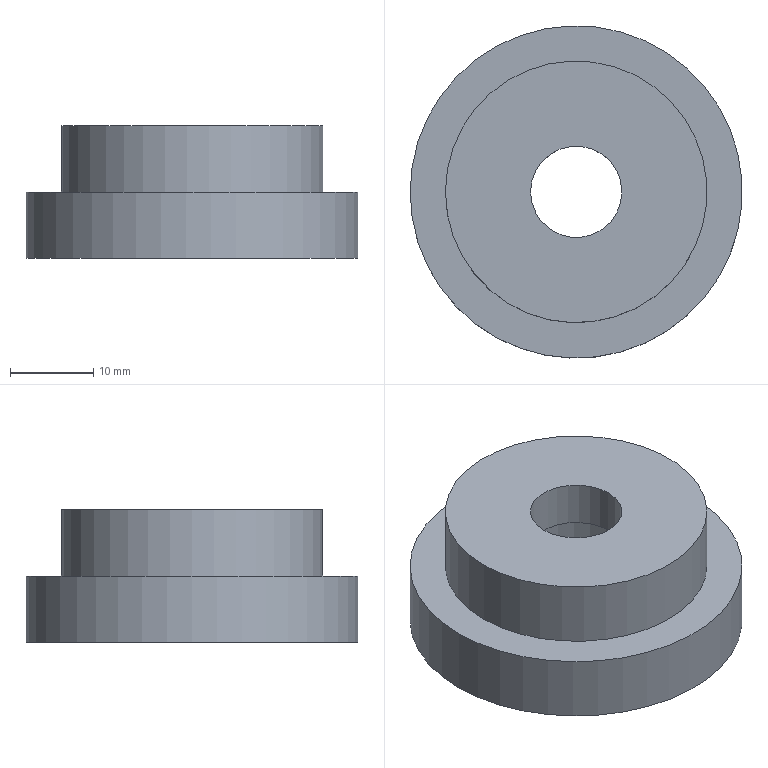Part | STEP file | PN_0057_id1206_x_t | 1 solid | 8 faces | box 40 x 40 x 16 mm | volume 13382 mm3 | cylinder 4 | plane 4 | commonest cylinder face diameters 11 x1 17 x1 31.5 x1 40 x1
STEP:
#1=CARTESIAN_POINT('',(232.,152.5,35.5));
#2=VERTEX_POINT('',#1);
#3=CARTESIAN_POINT('',(237.5,152.5,35.5));
#4=DIRECTION('',(0.,0.,-1.));
#5=DIRECTION('',(-1.,0.,0.));
#6=AXIS2_PLACEMENT_3D('',#3,#4,#5);
#7=CIRCLE('',#6,5.5);
#8=EDGE_CURVE('',#2,#2,#7,.T.);
#9=ORIENTED_EDGE('',*,*,#8,.T.);
#10=CARTESIAN_POINT('',(232.,152.5,41.));
#11=VERTEX_POINT('',#10);
#12=CARTESIAN_POINT('',(232.,152.5,35.5));
#13=CARTESIAN_POINT('',(232.,152.5,41.));
#14=B_SPLINE_CURVE_WITH_KNOTS('',1,(#12,#13),.UNSPECIFIED.,.F.,.F.,(2,2),(0.,1.),.UNSPECIFIED.);
#15=EDGE_CURVE('',#2,#11,#14,.T.);
#16=ORIENTED_EDGE('',*,*,#15,.T.);
#17=CARTESIAN_POINT('',(237.5,152.5,41.));
#18=DIRECTION('',(0.,0.,1.));
#19=DIRECTION('',(-1.,0.,0.));
#20=AXIS2_PLACEMENT_3D('',#17,#18,#19);
#21=CIRCLE('',#20,5.5);
#22=EDGE_CURVE('',#11,#11,#21,.T.);
#23=ORIENTED_EDGE('',*,*,#22,.T.);
#24=ORIENTED_EDGE('',*,*,#15,.F.);
#25=EDGE_LOOP('',(#9,#16,#23,#24));
#26=FACE_OUTER_BOUND('',#25,.T.);
#27=CARTESIAN_POINT('',(237.5,152.5,38.25));
#28=DIRECTION('',(0.,0.,1.));
#29=DIRECTION('',(-1.,0.,0.));
#30=AXIS2_PLACEMENT_3D('',#27,#28,#29);
#31=CYLINDRICAL_SURFACE('',#30,5.5);
#32=ADVANCED_FACE('',(#26),#31,.F.);
#33=CARTESIAN_POINT('',(229.,152.5,25.));
#34=VERTEX_POINT('',#33);
#35=CARTESIAN_POINT('',(237.5,152.5,25.));
#36=DIRECTION('',(0.,0.,-1.));
#37=DIRECTION('',(-1.,0.,0.));
#38=AXIS2_PLACEMENT_3D('',#35,#36,#37);
#39=CIRCLE('',#38,8.5);
#40=EDGE_CURVE('',#34,#34,#39,.T.);
#41=ORIENTED_EDGE('',*,*,#40,.T.);
#42=CARTESIAN_POINT('',(229.,152.5,35.5));
#43=VERTEX_POINT('',#42);
#44=CARTESIAN_POINT('',(229.,152.5,25.));
#45=CARTESIAN_POINT('',(229.,152.5,35.5));
#46=B_SPLINE_CURVE_WITH_KNOTS('',1,(#44,#45),.UNSPECIFIED.,.F.,.F.,(2,2),(0.,1.),.UNSPECIFIED.);
#47=EDGE_CURVE('',#34,#43,#46,.T.);
#48=ORIENTED_EDGE('',*,*,#47,.T.);
#49=CARTESIAN_POINT('',(237.5,152.5,35.5));
#50=DIRECTION('',(0.,0.,-1.));
#51=DIRECTION('',(-1.,0.,0.));
#52=AXIS2_PLACEMENT_3D('',#49,#50,#51);
#53=CIRCLE('',#52,8.5);
#54=EDGE_CURVE('',#43,#43,#53,.T.);
#55=ORIENTED_EDGE('',*,*,#54,.F.);
#56=ORIENTED_EDGE('',*,*,#47,.F.);
#57=EDGE_LOOP('',(#41,#48,#55,#56));
#58=FACE_OUTER_BOUND('',#57,.T.);
#59=CARTESIAN_POINT('',(237.5,152.5,30.25));
#60=DIRECTION('',(0.,0.,1.));
#61=DIRECTION('',(-1.,0.,0.));
#62=AXIS2_PLACEMENT_3D('',#59,#60,#61);
#63=CYLINDRICAL_SURFACE('',#62,8.5);
#64=ADVANCED_FACE('',(#58),#63,.F.);
#65=ORIENTED_EDGE('',*,*,#54,.T.);
#66=EDGE_LOOP('',(#65));
#67=FACE_BOUND('',#66,.T.);
#68=ORIENTED_EDGE('',*,*,#8,.F.);
#69=EDGE_LOOP('',(#68));
#70=FACE_BOUND('',#69,.T.);
#71=CARTESIAN_POINT('',(257.05,134.833,35.5));
#72=DIRECTION('',(0.,0.,1.));
#73=DIRECTION('',(-1.,0.,0.));
#74=AXIS2_PLACEMENT_3D('',#71,#72,#73);
#75=PLANE('',#74);
#76=ADVANCED_FACE('',(#67,#70),#75,.F.);
#77=CARTESIAN_POINT('',(221.75,152.5,33.));
#78=VERTEX_POINT('',#77);
#79=CARTESIAN_POINT('',(237.5,152.5,33.));
#80=DIRECTION('',(0.,0.,1.));
#81=DIRECTION('',(-1.,0.,0.));
#82=AXIS2_PLACEMENT_3D('',#79,#80,#81);
#83=CIRCLE('',#82,15.75);
#84=EDGE_CURVE('',#78,#78,#83,.T.);
#85=ORIENTED_EDGE('',*,*,#84,.T.);
#86=CARTESIAN_POINT('',(221.75,152.5,41.));
#87=VERTEX_POINT('',#86);
#88=CARTESIAN_POINT('',(221.75,152.5,33.));
#89=CARTESIAN_POINT('',(221.75,152.5,41.));
#90=B_SPLINE_CURVE_WITH_KNOTS('',1,(#88,#89),.UNSPECIFIED.,.F.,.F.,(2,2),(0.,1.),.UNSPECIFIED.);
#91=EDGE_CURVE('',#78,#87,#90,.T.);
#92=ORIENTED_EDGE('',*,*,#91,.T.);
#93=CARTESIAN_POINT('',(237.5,152.5,41.));
#94=DIRECTION('',(0.,0.,-1.));
#95=DIRECTION('',(-1.,0.,0.));
#96=AXIS2_PLACEMENT_3D('',#93,#94,#95);
#97=CIRCLE('',#96,15.75);
#98=EDGE_CURVE('',#87,#87,#97,.T.);
#99=ORIENTED_EDGE('',*,*,#98,.T.);
#100=ORIENTED_EDGE('',*,*,#91,.F.);
#101=EDGE_LOOP('',(#85,#92,#99,#100));
#102=FACE_OUTER_BOUND('',#101,.T.);
#103=CARTESIAN_POINT('',(237.5,152.5,37.));
#104=DIRECTION('',(0.,0.,1.));
#105=DIRECTION('',(-1.,0.,0.));
#106=AXIS2_PLACEMENT_3D('',#103,#104,#105);
#107=CYLINDRICAL_SURFACE('',#106,15.75);
#108=ADVANCED_FACE('',(#102),#107,.T.);
#109=ORIENTED_EDGE('',*,*,#98,.F.);
#110=EDGE_LOOP('',(#109));
#111=FACE_BOUND('',#110,.T.);
#112=ORIENTED_EDGE('',*,*,#22,.F.);
#113=EDGE_LOOP('',(#112));
#114=FACE_BOUND('',#113,.T.);
#115=CARTESIAN_POINT('',(273.725,119.764,41.));
#116=DIRECTION('',(0.,0.,1.));
#117=DIRECTION('',(-1.,0.,0.));
#118=AXIS2_PLACEMENT_3D('',#115,#116,#117);
#119=PLANE('',#118);
#120=ADVANCED_FACE('',(#111,#114),#119,.T.);
#121=CARTESIAN_POINT('',(217.5,152.5,25.));
#122=VERTEX_POINT('',#121);
#123=CARTESIAN_POINT('',(237.5,152.5,25.));
#124=DIRECTION('',(0.,0.,1.));
#125=DIRECTION('',(-1.,0.,0.));
#126=AXIS2_PLACEMENT_3D('',#123,#124,#125);
#127=CIRCLE('',#126,20.);
#128=EDGE_CURVE('',#122,#122,#127,.T.);
#129=ORIENTED_EDGE('',*,*,#128,.T.);
#130=CARTESIAN_POINT('',(217.5,152.5,33.));
#131=VERTEX_POINT('',#130);
#132=CARTESIAN_POINT('',(217.5,152.5,25.));
#133=CARTESIAN_POINT('',(217.5,152.5,33.));
#134=B_SPLINE_CURVE_WITH_KNOTS('',1,(#132,#133),.UNSPECIFIED.,.F.,.F.,(2,2),(0.,1.),.UNSPECIFIED.);
#135=EDGE_CURVE('',#122,#131,#134,.T.);
#136=ORIENTED_EDGE('',*,*,#135,.T.);
#137=CARTESIAN_POINT('',(237.5,152.5,33.));
#138=DIRECTION('',(0.,0.,-1.));
#139=DIRECTION('',(-1.,0.,0.));
#140=AXIS2_PLACEMENT_3D('',#137,#138,#139);
#141=CIRCLE('',#140,20.);
#142=EDGE_CURVE('',#131,#131,#141,.T.);
#143=ORIENTED_EDGE('',*,*,#142,.T.);
#144=ORIENTED_EDGE('',*,*,#135,.F.);
#145=EDGE_LOOP('',(#129,#136,#143,#144));
#146=FACE_OUTER_BOUND('',#145,.T.);
#147=CARTESIAN_POINT('',(237.5,152.5,29.));
#148=DIRECTION('',(0.,0.,1.));
#149=DIRECTION('',(-1.,0.,0.));
#150=AXIS2_PLACEMENT_3D('',#147,#148,#149);
#151=CYLINDRICAL_SURFACE('',#150,20.);
#152=ADVANCED_FACE('',(#146),#151,.T.);
#153=ORIENTED_EDGE('',*,*,#128,.F.);
#154=EDGE_LOOP('',(#153));
#155=FACE_BOUND('',#154,.T.);
#156=ORIENTED_EDGE('',*,*,#40,.F.);
#157=EDGE_LOOP('',(#156));
#158=FACE_BOUND('',#157,.T.);
#159=CARTESIAN_POINT('',(211.5,110.931,25.));
#160=DIRECTION('',(0.,0.,-1.));
#161=DIRECTION('',(1.,0.,0.));
#162=AXIS2_PLACEMENT_3D('',#159,#160,#161);
#163=PLANE('',#162);
#164=ADVANCED_FACE('',(#155,#158),#163,.T.);
#165=ORIENTED_EDGE('',*,*,#142,.F.);
#166=EDGE_LOOP('',(#165));
#167=FACE_BOUND('',#166,.T.);
#168=ORIENTED_EDGE('',*,*,#84,.F.);
#169=EDGE_LOOP('',(#168));
#170=FACE_BOUND('',#169,.T.);
#171=CARTESIAN_POINT('',(283.5,110.931,33.));
#172=DIRECTION('',(0.,0.,1.));
#173=DIRECTION('',(-1.,0.,0.));
#174=AXIS2_PLACEMENT_3D('',#171,#172,#173);
#175=PLANE('',#174);
#176=ADVANCED_FACE('',(#167,#170),#175,.T.);
#177=CLOSED_SHELL('',(#32,#64,#76,#108,#120,#152,#164,#176));
#178=MANIFOLD_SOLID_BREP('',#177);
#179=(LENGTH_UNIT()NAMED_UNIT(*)SI_UNIT(.MILLI.,.METRE.));
#180=UNCERTAINTY_MEASURE_WITH_UNIT(LENGTH_MEASURE(0.00002),#179,'','');
#181=(NAMED_UNIT(*)PLANE_ANGLE_UNIT()SI_UNIT($,.RADIAN.));
#182=PLANE_ANGLE_MEASURE_WITH_UNIT(PLANE_ANGLE_MEASURE(0.01745),#181);
#183=DIMENSIONAL_EXPONENTS(0.,0.,0.,0.,0.,0.,0.);
#184=(CONVERSION_BASED_UNIT('DEGREE',#182)NAMED_UNIT(#183)PLANE_ANGLE_UNIT());
#185=(NAMED_UNIT(*)SI_UNIT($,.STERADIAN.)SOLID_ANGLE_UNIT());
#186=(GEOMETRIC_REPRESENTATION_CONTEXT(3)GLOBAL_UNCERTAINTY_ASSIGNED_CONTEXT((#180))GLOBAL_UNIT_ASSIGNED_CONTEXT((#179,#184,#185))REPRESENTATION_CONTEXT('',''));
#187=ADVANCED_BREP_SHAPE_REPRESENTATION('',(#178),#186);